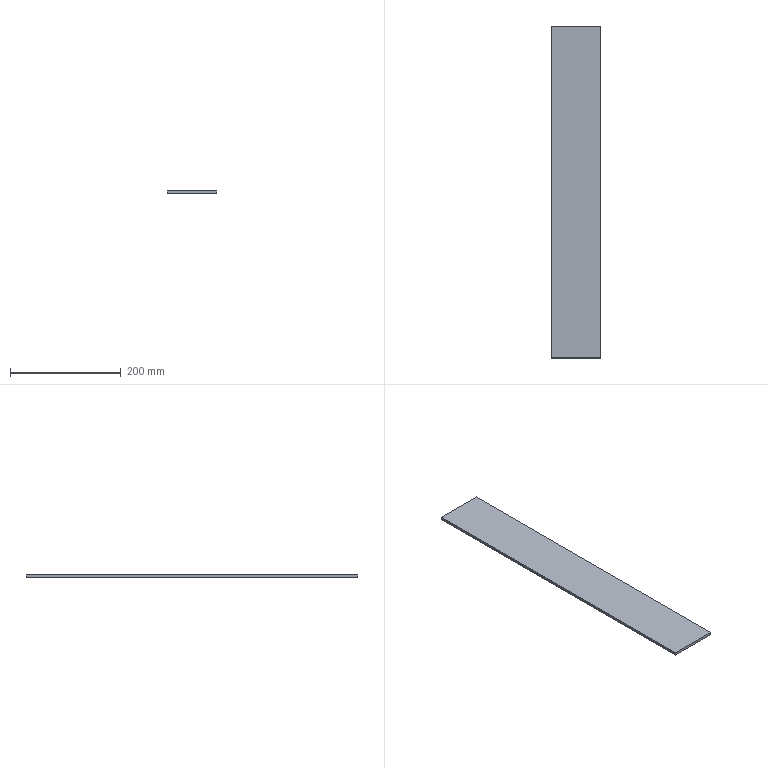Part | SolidWorks | features Extrusion 1, ICE 1 | 1 solid | 6 faces | box 90 x 600 x 5 mm | volume 270000 mm3 | plane 6
STEP:
#1=CARTESIAN_POINT('',(0.,0.,3.));
#2=VERTEX_POINT('',#1);
#3=CARTESIAN_POINT('',(0.,0.,-2.));
#4=VERTEX_POINT('',#3);
#5=CARTESIAN_POINT('',(0.,0.,3.));
#6=DIRECTION('',(0.,0.,-1.));
#7=VECTOR('',#6,1000.);
#8=LINE('',#5,#7);
#9=EDGE_CURVE('',#2,#4,#8,.T.);
#10=ORIENTED_EDGE('',*,*,#9,.T.);
#11=CARTESIAN_POINT('',(90.,0.,-2.));
#12=VERTEX_POINT('',#11);
#13=CARTESIAN_POINT('',(90.,0.,-2.));
#14=DIRECTION('',(-1.,0.,0.));
#15=VECTOR('',#14,1000.);
#16=LINE('',#13,#15);
#17=EDGE_CURVE('',#12,#4,#16,.T.);
#18=ORIENTED_EDGE('',*,*,#17,.F.);
#19=CARTESIAN_POINT('',(90.,0.,3.));
#20=VERTEX_POINT('',#19);
#21=CARTESIAN_POINT('',(90.,0.,3.));
#22=DIRECTION('',(0.,0.,-1.));
#23=VECTOR('',#22,1000.);
#24=LINE('',#21,#23);
#25=EDGE_CURVE('',#20,#12,#24,.T.);
#26=ORIENTED_EDGE('',*,*,#25,.F.);
#27=CARTESIAN_POINT('',(90.,0.,3.));
#28=DIRECTION('',(1.,0.,0.));
#29=VECTOR('',#28,1000.);
#30=LINE('',#27,#29);
#31=EDGE_CURVE('',#2,#20,#30,.T.);
#32=ORIENTED_EDGE('',*,*,#31,.F.);
#33=EDGE_LOOP('',(#10,#18,#26,#32));
#34=FACE_OUTER_BOUND('',#33,.T.);
#35=CARTESIAN_POINT('',(90.,0.,3.));
#36=DIRECTION('',(0.,1.,0.));
#37=DIRECTION('',(0.,0.,1.));
#38=AXIS2_PLACEMENT_3D('',#35,#36,#37);
#39=PLANE('',#38);
#40=ADVANCED_FACE('',(#34),#39,.F.);
#41=ORIENTED_EDGE('',*,*,#25,.T.);
#42=CARTESIAN_POINT('',(90.,600.,-2.));
#43=VERTEX_POINT('',#42);
#44=CARTESIAN_POINT('',(90.,600.,-2.));
#45=DIRECTION('',(0.,-1.,0.));
#46=VECTOR('',#45,1000.);
#47=LINE('',#44,#46);
#48=EDGE_CURVE('',#43,#12,#47,.T.);
#49=ORIENTED_EDGE('',*,*,#48,.F.);
#50=CARTESIAN_POINT('',(90.,600.,3.));
#51=VERTEX_POINT('',#50);
#52=CARTESIAN_POINT('',(90.,600.,3.));
#53=DIRECTION('',(0.,0.,-1.));
#54=VECTOR('',#53,1000.);
#55=LINE('',#52,#54);
#56=EDGE_CURVE('',#51,#43,#55,.T.);
#57=ORIENTED_EDGE('',*,*,#56,.F.);
#58=CARTESIAN_POINT('',(90.,600.,3.));
#59=DIRECTION('',(0.,1.,0.));
#60=VECTOR('',#59,1000.);
#61=LINE('',#58,#60);
#62=EDGE_CURVE('',#20,#51,#61,.T.);
#63=ORIENTED_EDGE('',*,*,#62,.F.);
#64=EDGE_LOOP('',(#41,#49,#57,#63));
#65=FACE_OUTER_BOUND('',#64,.T.);
#66=CARTESIAN_POINT('',(90.,600.,3.));
#67=DIRECTION('',(-1.,0.,0.));
#68=DIRECTION('',(0.,0.,1.));
#69=AXIS2_PLACEMENT_3D('',#66,#67,#68);
#70=PLANE('',#69);
#71=ADVANCED_FACE('',(#65),#70,.F.);
#72=ORIENTED_EDGE('',*,*,#56,.T.);
#73=CARTESIAN_POINT('',(0.,600.,-2.));
#74=VERTEX_POINT('',#73);
#75=CARTESIAN_POINT('',(0.,600.,-2.));
#76=DIRECTION('',(1.,0.,0.));
#77=VECTOR('',#76,1000.);
#78=LINE('',#75,#77);
#79=EDGE_CURVE('',#74,#43,#78,.T.);
#80=ORIENTED_EDGE('',*,*,#79,.F.);
#81=CARTESIAN_POINT('',(0.,600.,3.));
#82=VERTEX_POINT('',#81);
#83=CARTESIAN_POINT('',(0.,600.,3.));
#84=DIRECTION('',(0.,0.,-1.));
#85=VECTOR('',#84,1000.);
#86=LINE('',#83,#85);
#87=EDGE_CURVE('',#82,#74,#86,.T.);
#88=ORIENTED_EDGE('',*,*,#87,.F.);
#89=CARTESIAN_POINT('',(0.,600.,3.));
#90=DIRECTION('',(-1.,0.,0.));
#91=VECTOR('',#90,1000.);
#92=LINE('',#89,#91);
#93=EDGE_CURVE('',#51,#82,#92,.T.);
#94=ORIENTED_EDGE('',*,*,#93,.F.);
#95=EDGE_LOOP('',(#72,#80,#88,#94));
#96=FACE_OUTER_BOUND('',#95,.T.);
#97=CARTESIAN_POINT('',(0.,600.,3.));
#98=DIRECTION('',(0.,-1.,0.));
#99=DIRECTION('',(0.,0.,-1.));
#100=AXIS2_PLACEMENT_3D('',#97,#98,#99);
#101=PLANE('',#100);
#102=ADVANCED_FACE('',(#96),#101,.F.);
#103=ORIENTED_EDGE('',*,*,#87,.T.);
#104=CARTESIAN_POINT('',(0.,0.,-2.));
#105=DIRECTION('',(0.,1.,0.));
#106=VECTOR('',#105,1000.);
#107=LINE('',#104,#106);
#108=EDGE_CURVE('',#4,#74,#107,.T.);
#109=ORIENTED_EDGE('',*,*,#108,.F.);
#110=ORIENTED_EDGE('',*,*,#9,.F.);
#111=CARTESIAN_POINT('',(0.,0.,3.));
#112=DIRECTION('',(0.,-1.,0.));
#113=VECTOR('',#112,1000.);
#114=LINE('',#111,#113);
#115=EDGE_CURVE('',#82,#2,#114,.T.);
#116=ORIENTED_EDGE('',*,*,#115,.F.);
#117=EDGE_LOOP('',(#103,#109,#110,#116));
#118=FACE_OUTER_BOUND('',#117,.T.);
#119=CARTESIAN_POINT('',(0.,0.,3.));
#120=DIRECTION('',(1.,0.,0.));
#121=DIRECTION('',(0.,0.,-1.));
#122=AXIS2_PLACEMENT_3D('',#119,#120,#121);
#123=PLANE('',#122);
#124=ADVANCED_FACE('',(#118),#123,.F.);
#125=ORIENTED_EDGE('',*,*,#31,.T.);
#126=ORIENTED_EDGE('',*,*,#62,.T.);
#127=ORIENTED_EDGE('',*,*,#93,.T.);
#128=ORIENTED_EDGE('',*,*,#115,.T.);
#129=EDGE_LOOP('',(#125,#126,#127,#128));
#130=FACE_OUTER_BOUND('',#129,.T.);
#131=CARTESIAN_POINT('',(0.,0.,3.));
#132=DIRECTION('',(0.,0.,-1.));
#133=DIRECTION('',(-1.,0.,0.));
#134=AXIS2_PLACEMENT_3D('',#131,#132,#133);
#135=PLANE('',#134);
#136=ADVANCED_FACE('',(#130),#135,.F.);
#137=ORIENTED_EDGE('',*,*,#48,.T.);
#138=ORIENTED_EDGE('',*,*,#17,.T.);
#139=ORIENTED_EDGE('',*,*,#108,.T.);
#140=ORIENTED_EDGE('',*,*,#79,.T.);
#141=EDGE_LOOP('',(#137,#138,#139,#140));
#142=FACE_OUTER_BOUND('',#141,.T.);
#143=CARTESIAN_POINT('',(0.,0.,-2.));
#144=DIRECTION('',(0.,0.,-1.));
#145=DIRECTION('',(-1.,0.,0.));
#146=AXIS2_PLACEMENT_3D('',#143,#144,#145);
#147=PLANE('',#146);
#148=ADVANCED_FACE('',(#142),#147,.T.);
#149=CLOSED_SHELL('',(#40,#71,#102,#124,#136,#148));
#150=MANIFOLD_SOLID_BREP('',#149);
#151=CARTESIAN_POINT('',(0.,0.,0.));
#152=DIRECTION('',(0.,0.,1.));
#153=DIRECTION('',(1.,0.,0.));
#154=AXIS2_PLACEMENT_3D('',#151,#152,#153);
#155=(LENGTH_UNIT()NAMED_UNIT(*)SI_UNIT(.MILLI.,.METRE.));
#156=UNCERTAINTY_MEASURE_WITH_UNIT(LENGTH_MEASURE(0.00001),#155,'','');
#157=(NAMED_UNIT(*)PLANE_ANGLE_UNIT()SI_UNIT($,.RADIAN.));
#158=(NAMED_UNIT(*)SI_UNIT($,.STERADIAN.)SOLID_ANGLE_UNIT());
#159=(GEOMETRIC_REPRESENTATION_CONTEXT(3)GLOBAL_UNCERTAINTY_ASSIGNED_CONTEXT((#156))GLOBAL_UNIT_ASSIGNED_CONTEXT((#155,#157,#158))REPRESENTATION_CONTEXT('',''));
#160=ADVANCED_BREP_SHAPE_REPRESENTATION('',(#150,#154),#159);